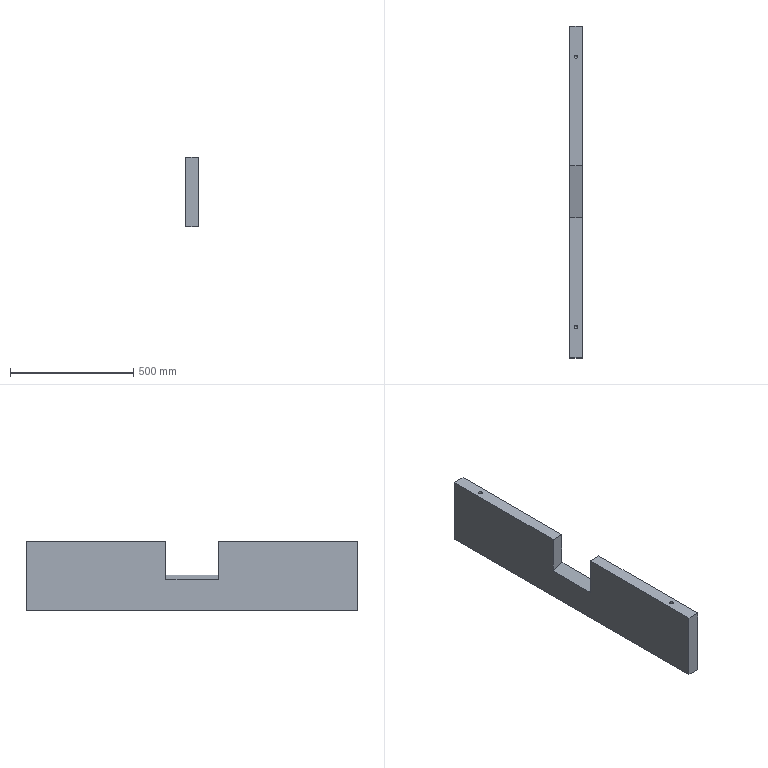Part | NX | features 29 2 | 1 solid | 20 faces | box 50 x 1345 x 280.5 mm | volume 17283100 mm3 | plane 10 | cylinder 5 | cone 5 | commonest cylinder face diameters 14.1 x5
STEP:
#1=CARTESIAN_POINT('',(3647.05,-547.5,-493.5));
#2=VERTEX_POINT('',#1);
#3=CARTESIAN_POINT('',(3640.,-547.5,-493.5));
#4=DIRECTION('',(0.,0.,1.));
#5=DIRECTION('',(1.,0.,0.));
#6=AXIS2_PLACEMENT_3D('',#3,#4,#5);
#7=CIRCLE('',#6,7.05);
#8=EDGE_CURVE('',#2,#2,#7,.T.);
#9=ORIENTED_EDGE('',*,*,#8,.T.);
#10=EDGE_LOOP('',(#9));
#11=FACE_BOUND('',#10,.T.);
#12=CARTESIAN_POINT('',(3615.,672.5,-493.5));
#13=VERTEX_POINT('',#12);
#14=CARTESIAN_POINT('',(3615.,-672.5,-493.5));
#15=VERTEX_POINT('',#14);
#16=CARTESIAN_POINT('',(3615.,193.,-493.5));
#17=DIRECTION('',(0.,-1.,0.));
#18=VECTOR('',#17,1000.);
#19=LINE('',#16,#18);
#20=EDGE_CURVE('',#13,#15,#19,.T.);
#21=ORIENTED_EDGE('',*,*,#20,.F.);
#22=CARTESIAN_POINT('',(3665.,672.5,-493.5));
#23=VERTEX_POINT('',#22);
#24=CARTESIAN_POINT('',(1502.5,672.5,-493.5));
#25=DIRECTION('',(1.,0.,0.));
#26=VECTOR('',#25,1000.);
#27=LINE('',#24,#26);
#28=EDGE_CURVE('',#13,#23,#27,.T.);
#29=ORIENTED_EDGE('',*,*,#28,.T.);
#30=CARTESIAN_POINT('',(3665.,-672.5,-493.5));
#31=VERTEX_POINT('',#30);
#32=CARTESIAN_POINT('',(3665.,193.,-493.5));
#33=DIRECTION('',(0.,1.,0.));
#34=VECTOR('',#33,1000.);
#35=LINE('',#32,#34);
#36=EDGE_CURVE('',#31,#23,#35,.T.);
#37=ORIENTED_EDGE('',*,*,#36,.F.);
#38=CARTESIAN_POINT('',(4005.,-672.5,-493.5));
#39=DIRECTION('',(-1.,0.,0.));
#40=VECTOR('',#39,1000.);
#41=LINE('',#38,#40);
#42=EDGE_CURVE('',#31,#15,#41,.T.);
#43=ORIENTED_EDGE('',*,*,#42,.T.);
#44=EDGE_LOOP('',(#21,#29,#37,#43));
#45=FACE_BOUND('',#44,.T.);
#46=CARTESIAN_POINT('',(3647.05,547.5,-493.5));
#47=VERTEX_POINT('',#46);
#48=CARTESIAN_POINT('',(3640.,547.5,-493.5));
#49=DIRECTION('',(0.,0.,1.));
#50=DIRECTION('',(1.,0.,0.));
#51=AXIS2_PLACEMENT_3D('',#48,#49,#50);
#52=CIRCLE('',#51,7.05);
#53=EDGE_CURVE('',#47,#47,#52,.T.);
#54=ORIENTED_EDGE('',*,*,#53,.T.);
#55=EDGE_LOOP('',(#54));
#56=FACE_BOUND('',#55,.T.);
#57=CARTESIAN_POINT('',(3647.05,0.,-493.5));
#58=VERTEX_POINT('',#57);
#59=CARTESIAN_POINT('',(3640.,0.,-493.5));
#60=DIRECTION('',(0.,0.,1.));
#61=DIRECTION('',(1.,0.,0.));
#62=AXIS2_PLACEMENT_3D('',#59,#60,#61);
#63=CIRCLE('',#62,7.05);
#64=EDGE_CURVE('',#58,#58,#63,.T.);
#65=ORIENTED_EDGE('',*,*,#64,.T.);
#66=EDGE_LOOP('',(#65));
#67=FACE_BOUND('',#66,.T.);
#68=CARTESIAN_POINT('',(1945.,0.,-493.5));
#69=DIRECTION('',(0.,0.,-1.));
#70=DIRECTION('',(1.,0.,0.));
#71=AXIS2_PLACEMENT_3D('',#68,#69,#70);
#72=PLANE('',#71);
#73=ADVANCED_FACE('',(#11,#45,#56,#67),#72,.T.);
#74=CARTESIAN_POINT('',(3665.,-105.579,-213.));
#75=VERTEX_POINT('',#74);
#76=CARTESIAN_POINT('',(3615.,-105.579,-213.));
#77=VERTEX_POINT('',#76);
#78=CARTESIAN_POINT('',(1945.,-105.579,-213.));
#79=DIRECTION('',(-1.,0.,0.));
#80=VECTOR('',#79,1000.);
#81=LINE('',#78,#80);
#82=EDGE_CURVE('',#75,#77,#81,.T.);
#83=ORIENTED_EDGE('',*,*,#82,.T.);
#84=CARTESIAN_POINT('',(3615.,-672.5,-213.));
#85=VERTEX_POINT('',#84);
#86=CARTESIAN_POINT('',(3615.,193.,-213.));
#87=DIRECTION('',(0.,1.,0.));
#88=VECTOR('',#87,1000.);
#89=LINE('',#86,#88);
#90=EDGE_CURVE('',#85,#77,#89,.T.);
#91=ORIENTED_EDGE('',*,*,#90,.F.);
#92=CARTESIAN_POINT('',(3665.,-672.5,-213.));
#93=VERTEX_POINT('',#92);
#94=CARTESIAN_POINT('',(4005.,-672.5,-213.));
#95=DIRECTION('',(1.,0.,0.));
#96=VECTOR('',#95,1000.);
#97=LINE('',#94,#96);
#98=EDGE_CURVE('',#85,#93,#97,.T.);
#99=ORIENTED_EDGE('',*,*,#98,.T.);
#100=CARTESIAN_POINT('',(3665.,193.,-213.));
#101=DIRECTION('',(0.,-1.,0.));
#102=VECTOR('',#101,1000.);
#103=LINE('',#100,#102);
#104=EDGE_CURVE('',#75,#93,#103,.T.);
#105=ORIENTED_EDGE('',*,*,#104,.F.);
#106=EDGE_LOOP('',(#83,#91,#99,#105));
#107=FACE_BOUND('',#106,.T.);
#108=CARTESIAN_POINT('',(3647.05,-547.5,-213.));
#109=VERTEX_POINT('',#108);
#110=CARTESIAN_POINT('',(3640.,-547.5,-213.));
#111=DIRECTION('',(0.,0.,-1.));
#112=DIRECTION('',(1.,0.,0.));
#113=AXIS2_PLACEMENT_3D('',#110,#111,#112);
#114=CIRCLE('',#113,7.05);
#115=EDGE_CURVE('',#109,#109,#114,.T.);
#116=ORIENTED_EDGE('',*,*,#115,.T.);
#117=EDGE_LOOP('',(#116));
#118=FACE_BOUND('',#117,.T.);
#119=CARTESIAN_POINT('',(1945.,0.,-213.));
#120=DIRECTION('',(0.,0.,1.));
#121=DIRECTION('',(-1.,0.,0.));
#122=AXIS2_PLACEMENT_3D('',#119,#120,#121);
#123=PLANE('',#122);
#124=ADVANCED_FACE('',(#107,#118),#123,.T.);
#125=CARTESIAN_POINT('',(3665.,105.421,-213.));
#126=VERTEX_POINT('',#125);
#127=CARTESIAN_POINT('',(3615.,105.421,-213.));
#128=VERTEX_POINT('',#127);
#129=CARTESIAN_POINT('',(3821.81,105.421,-213.));
#130=DIRECTION('',(-1.,0.,0.));
#131=VECTOR('',#130,1000.);
#132=LINE('',#129,#131);
#133=EDGE_CURVE('',#126,#128,#132,.T.);
#134=ORIENTED_EDGE('',*,*,#133,.F.);
#135=CARTESIAN_POINT('',(3665.,672.5,-213.));
#136=VERTEX_POINT('',#135);
#137=CARTESIAN_POINT('',(3665.,193.,-213.));
#138=DIRECTION('',(0.,-1.,0.));
#139=VECTOR('',#138,1000.);
#140=LINE('',#137,#139);
#141=EDGE_CURVE('',#136,#126,#140,.T.);
#142=ORIENTED_EDGE('',*,*,#141,.F.);
#143=CARTESIAN_POINT('',(3615.,672.5,-213.));
#144=VERTEX_POINT('',#143);
#145=CARTESIAN_POINT('',(1502.5,672.5,-213.));
#146=DIRECTION('',(-1.,0.,0.));
#147=VECTOR('',#146,1000.);
#148=LINE('',#145,#147);
#149=EDGE_CURVE('',#136,#144,#148,.T.);
#150=ORIENTED_EDGE('',*,*,#149,.T.);
#151=CARTESIAN_POINT('',(3615.,193.,-213.));
#152=DIRECTION('',(0.,1.,0.));
#153=VECTOR('',#152,1000.);
#154=LINE('',#151,#153);
#155=EDGE_CURVE('',#128,#144,#154,.T.);
#156=ORIENTED_EDGE('',*,*,#155,.F.);
#157=EDGE_LOOP('',(#134,#142,#150,#156));
#158=FACE_BOUND('',#157,.T.);
#159=CARTESIAN_POINT('',(3647.05,547.5,-213.));
#160=VERTEX_POINT('',#159);
#161=CARTESIAN_POINT('',(3640.,547.5,-213.));
#162=DIRECTION('',(0.,0.,-1.));
#163=DIRECTION('',(1.,0.,0.));
#164=AXIS2_PLACEMENT_3D('',#161,#162,#163);
#165=CIRCLE('',#164,7.05);
#166=EDGE_CURVE('',#160,#160,#165,.T.);
#167=ORIENTED_EDGE('',*,*,#166,.T.);
#168=EDGE_LOOP('',(#167));
#169=FACE_BOUND('',#168,.T.);
#170=CARTESIAN_POINT('',(1945.,0.,-213.));
#171=DIRECTION('',(0.,0.,1.));
#172=DIRECTION('',(-1.,0.,0.));
#173=AXIS2_PLACEMENT_3D('',#170,#171,#172);
#174=PLANE('',#173);
#175=ADVANCED_FACE('',(#158,#169),#174,.T.);
#176=ORIENTED_EDGE('',*,*,#90,.T.);
#177=CARTESIAN_POINT('',(3615.,-105.579,-369.004));
#178=VERTEX_POINT('',#177);
#179=CARTESIAN_POINT('',(3615.,-105.579,-205.5));
#180=DIRECTION('',(0.,0.,-1.));
#181=VECTOR('',#180,1000.);
#182=LINE('',#179,#181);
#183=EDGE_CURVE('',#77,#178,#182,.T.);
#184=ORIENTED_EDGE('',*,*,#183,.T.);
#185=CARTESIAN_POINT('',(3615.,105.421,-369.004));
#186=VERTEX_POINT('',#185);
#187=CARTESIAN_POINT('',(3615.,193.,-369.004));
#188=DIRECTION('',(0.,1.,0.));
#189=VECTOR('',#188,1000.);
#190=LINE('',#187,#189);
#191=EDGE_CURVE('',#178,#186,#190,.T.);
#192=ORIENTED_EDGE('',*,*,#191,.T.);
#193=CARTESIAN_POINT('',(3615.,105.421,-205.5));
#194=DIRECTION('',(0.,0.,1.));
#195=VECTOR('',#194,1000.);
#196=LINE('',#193,#195);
#197=EDGE_CURVE('',#186,#128,#196,.T.);
#198=ORIENTED_EDGE('',*,*,#197,.T.);
#199=ORIENTED_EDGE('',*,*,#155,.T.);
#200=CARTESIAN_POINT('',(3615.,672.5,-205.5));
#201=DIRECTION('',(0.,0.,1.));
#202=VECTOR('',#201,1000.);
#203=LINE('',#200,#202);
#204=EDGE_CURVE('',#13,#144,#203,.T.);
#205=ORIENTED_EDGE('',*,*,#204,.F.);
#206=ORIENTED_EDGE('',*,*,#20,.T.);
#207=CARTESIAN_POINT('',(3615.,-672.5,-113.));
#208=DIRECTION('',(0.,0.,1.));
#209=VECTOR('',#208,1000.);
#210=LINE('',#207,#209);
#211=EDGE_CURVE('',#15,#85,#210,.T.);
#212=ORIENTED_EDGE('',*,*,#211,.T.);
#213=EDGE_LOOP('',(#176,#184,#192,#198,#199,#205,#206,#212));
#214=FACE_BOUND('',#213,.T.);
#215=CARTESIAN_POINT('',(3615.,193.,-205.5));
#216=DIRECTION('',(-1.,0.,0.));
#217=DIRECTION('',(0.,0.,1.));
#218=AXIS2_PLACEMENT_3D('',#215,#216,#217);
#219=PLANE('',#218);
#220=ADVANCED_FACE('',(#214),#219,.T.);
#221=ORIENTED_EDGE('',*,*,#28,.F.);
#222=ORIENTED_EDGE('',*,*,#204,.T.);
#223=ORIENTED_EDGE('',*,*,#149,.F.);
#224=CARTESIAN_POINT('',(3665.,672.5,-205.5));
#225=DIRECTION('',(0.,0.,1.));
#226=VECTOR('',#225,1000.);
#227=LINE('',#224,#226);
#228=EDGE_CURVE('',#23,#136,#227,.T.);
#229=ORIENTED_EDGE('',*,*,#228,.F.);
#230=EDGE_LOOP('',(#221,#222,#223,#229));
#231=FACE_BOUND('',#230,.T.);
#232=CARTESIAN_POINT('',(1502.5,672.5,91.));
#233=DIRECTION('',(0.,-1.,0.));
#234=DIRECTION('',(-1.,0.,0.));
#235=AXIS2_PLACEMENT_3D('',#232,#233,#234);
#236=PLANE('',#235);
#237=ADVANCED_FACE('',(#231),#236,.F.);
#238=CARTESIAN_POINT('',(3665.,-105.579,-350.805));
#239=VERTEX_POINT('',#238);
#240=CARTESIAN_POINT('',(3665.,-105.579,-205.5));
#241=DIRECTION('',(0.,0.,1.));
#242=VECTOR('',#241,1000.);
#243=LINE('',#240,#242);
#244=EDGE_CURVE('',#239,#75,#243,.T.);
#245=ORIENTED_EDGE('',*,*,#244,.T.);
#246=ORIENTED_EDGE('',*,*,#104,.T.);
#247=CARTESIAN_POINT('',(3665.,-672.5,-543.5));
#248=DIRECTION('',(0.,0.,1.));
#249=VECTOR('',#248,1000.);
#250=LINE('',#247,#249);
#251=EDGE_CURVE('',#31,#93,#250,.T.);
#252=ORIENTED_EDGE('',*,*,#251,.F.);
#253=ORIENTED_EDGE('',*,*,#36,.T.);
#254=ORIENTED_EDGE('',*,*,#228,.T.);
#255=ORIENTED_EDGE('',*,*,#141,.T.);
#256=CARTESIAN_POINT('',(3665.,105.421,-350.805));
#257=VERTEX_POINT('',#256);
#258=CARTESIAN_POINT('',(3665.,105.421,-205.5));
#259=DIRECTION('',(0.,0.,-1.));
#260=VECTOR('',#259,1000.);
#261=LINE('',#258,#260);
#262=EDGE_CURVE('',#126,#257,#261,.T.);
#263=ORIENTED_EDGE('',*,*,#262,.T.);
#264=CARTESIAN_POINT('',(3665.,193.,-350.805));
#265=DIRECTION('',(0.,-1.,0.));
#266=VECTOR('',#265,1000.);
#267=LINE('',#264,#266);
#268=EDGE_CURVE('',#257,#239,#267,.T.);
#269=ORIENTED_EDGE('',*,*,#268,.T.);
#270=EDGE_LOOP('',(#245,#246,#252,#253,#254,#255,#263,#269));
#271=FACE_BOUND('',#270,.T.);
#272=CARTESIAN_POINT('',(3665.,193.,-205.5));
#273=DIRECTION('',(1.,0.,0.));
#274=DIRECTION('',(0.,0.,-1.));
#275=AXIS2_PLACEMENT_3D('',#272,#273,#274);
#276=PLANE('',#275);
#277=ADVANCED_FACE('',(#271),#276,.T.);
#278=ORIENTED_EDGE('',*,*,#42,.F.);
#279=ORIENTED_EDGE('',*,*,#251,.T.);
#280=ORIENTED_EDGE('',*,*,#98,.F.);
#281=ORIENTED_EDGE('',*,*,#211,.F.);
#282=EDGE_LOOP('',(#278,#279,#280,#281));
#283=FACE_BOUND('',#282,.T.);
#284=CARTESIAN_POINT('',(4005.,-672.5,-113.));
#285=DIRECTION('',(0.,1.,0.));
#286=DIRECTION('',(1.,0.,0.));
#287=AXIS2_PLACEMENT_3D('',#284,#285,#286);
#288=PLANE('',#287);
#289=ADVANCED_FACE('',(#283),#288,.F.);
#290=ORIENTED_EDGE('',*,*,#82,.F.);
#291=ORIENTED_EDGE('',*,*,#244,.F.);
#292=CARTESIAN_POINT('',(3822.494,-105.579,-293.482));
#293=DIRECTION('',(0.9397,0.,0.342));
#294=VECTOR('',#293,1000.);
#295=LINE('',#292,#294);
#296=EDGE_CURVE('',#178,#239,#295,.T.);
#297=ORIENTED_EDGE('',*,*,#296,.F.);
#298=ORIENTED_EDGE('',*,*,#183,.F.);
#299=EDGE_LOOP('',(#290,#291,#297,#298));
#300=FACE_BOUND('',#299,.T.);
#301=CARTESIAN_POINT('',(3821.81,-105.579,-291.603));
#302=DIRECTION('',(0.,1.,0.));
#303=DIRECTION('',(-0.08716,0.,-0.9962));
#304=AXIS2_PLACEMENT_3D('',#301,#302,#303);
#305=PLANE('',#304);
#306=ADVANCED_FACE('',(#300),#305,.T.);
#307=ORIENTED_EDGE('',*,*,#296,.T.);
#308=ORIENTED_EDGE('',*,*,#268,.F.);
#309=CARTESIAN_POINT('',(3822.494,105.421,-293.482));
#310=DIRECTION('',(-0.9397,0.,-0.342));
#311=VECTOR('',#310,1000.);
#312=LINE('',#309,#311);
#313=EDGE_CURVE('',#257,#186,#312,.T.);
#314=ORIENTED_EDGE('',*,*,#313,.T.);
#315=ORIENTED_EDGE('',*,*,#191,.F.);
#316=EDGE_LOOP('',(#307,#308,#314,#315));
#317=FACE_BOUND('',#316,.T.);
#318=CARTESIAN_POINT('',(3822.494,-103.579,-293.482));
#319=DIRECTION('',(-0.342,0.,0.9397));
#320=DIRECTION('',(0.,1.,0.));
#321=AXIS2_PLACEMENT_3D('',#318,#319,#320);
#322=PLANE('',#321);
#323=ADVANCED_FACE('',(#317),#322,.T.);
#324=ORIENTED_EDGE('',*,*,#313,.F.);
#325=ORIENTED_EDGE('',*,*,#262,.F.);
#326=ORIENTED_EDGE('',*,*,#133,.T.);
#327=ORIENTED_EDGE('',*,*,#197,.F.);
#328=EDGE_LOOP('',(#324,#325,#326,#327));
#329=FACE_BOUND('',#328,.T.);
#330=CARTESIAN_POINT('',(3821.81,105.421,-291.603));
#331=DIRECTION('',(0.,-1.,0.));
#332=DIRECTION('',(0.08716,0.,0.9962));
#333=AXIS2_PLACEMENT_3D('',#330,#331,#332);
#334=PLANE('',#333);
#335=ADVANCED_FACE('',(#329),#334,.T.);
#336=CARTESIAN_POINT('',(3632.95,547.5,-249.95));
#337=VERTEX_POINT('',#336);
#338=CARTESIAN_POINT('',(3640.,547.5,-249.95));
#339=DIRECTION('',(0.,0.,-1.));
#340=DIRECTION('',(-1.,0.,0.));
#341=AXIS2_PLACEMENT_3D('',#338,#339,#340);
#342=CIRCLE('',#341,7.05);
#343=EDGE_CURVE('',#337,#337,#342,.T.);
#344=ORIENTED_EDGE('',*,*,#343,.T.);
#345=EDGE_LOOP('',(#344));
#346=FACE_BOUND('',#345,.T.);
#347=ORIENTED_EDGE('',*,*,#166,.F.);
#348=EDGE_LOOP('',(#347));
#349=FACE_BOUND('',#348,.T.);
#350=CARTESIAN_POINT('',(3640.,547.5,-213.));
#351=DIRECTION('',(0.,0.,-1.));
#352=DIRECTION('',(-1.,0.,0.));
#353=AXIS2_PLACEMENT_3D('',#350,#351,#352);
#354=CYLINDRICAL_SURFACE('',#353,7.05);
#355=ADVANCED_FACE('',(#346,#349),#354,.F.);
#356=CARTESIAN_POINT('',(3640.,547.5,-257.));
#357=VERTEX_POINT('',#356);
#358=VERTEX_LOOP('',#357);
#359=FACE_BOUND('',#358,.T.);
#360=ORIENTED_EDGE('',*,*,#343,.F.);
#361=EDGE_LOOP('',(#360));
#362=FACE_BOUND('',#361,.T.);
#363=CARTESIAN_POINT('',(3640.,547.5,-249.95));
#364=DIRECTION('',(0.,0.,1.));
#365=DIRECTION('',(-1.,0.,0.));
#366=AXIS2_PLACEMENT_3D('',#363,#364,#365);
#367=CONICAL_SURFACE('',#366,7.05,0.7854);
#368=ADVANCED_FACE('',(#359,#362),#367,.F.);
#369=CARTESIAN_POINT('',(3632.95,-547.5,-249.95));
#370=VERTEX_POINT('',#369);
#371=CARTESIAN_POINT('',(3640.,-547.5,-249.95));
#372=DIRECTION('',(0.,0.,-1.));
#373=DIRECTION('',(-1.,0.,0.));
#374=AXIS2_PLACEMENT_3D('',#371,#372,#373);
#375=CIRCLE('',#374,7.05);
#376=EDGE_CURVE('',#370,#370,#375,.T.);
#377=ORIENTED_EDGE('',*,*,#376,.T.);
#378=EDGE_LOOP('',(#377));
#379=FACE_BOUND('',#378,.T.);
#380=ORIENTED_EDGE('',*,*,#115,.F.);
#381=EDGE_LOOP('',(#380));
#382=FACE_BOUND('',#381,.T.);
#383=CARTESIAN_POINT('',(3640.,-547.5,-213.));
#384=DIRECTION('',(0.,0.,-1.));
#385=DIRECTION('',(-1.,0.,0.));
#386=AXIS2_PLACEMENT_3D('',#383,#384,#385);
#387=CYLINDRICAL_SURFACE('',#386,7.05);
#388=ADVANCED_FACE('',(#379,#382),#387,.F.);
#389=CARTESIAN_POINT('',(3640.,-547.5,-257.));
#390=VERTEX_POINT('',#389);
#391=VERTEX_LOOP('',#390);
#392=FACE_BOUND('',#391,.T.);
#393=ORIENTED_EDGE('',*,*,#376,.F.);
#394=EDGE_LOOP('',(#393));
#395=FACE_BOUND('',#394,.T.);
#396=CARTESIAN_POINT('',(3640.,-547.5,-249.95));
#397=DIRECTION('',(0.,0.,1.));
#398=DIRECTION('',(-1.,0.,0.));
#399=AXIS2_PLACEMENT_3D('',#396,#397,#398);
#400=CONICAL_SURFACE('',#399,7.05,0.7854);
#401=ADVANCED_FACE('',(#392,#395),#400,.F.);
#402=CARTESIAN_POINT('',(3647.05,547.5,-456.55));
#403=VERTEX_POINT('',#402);
#404=CARTESIAN_POINT('',(3640.,547.5,-456.55));
#405=DIRECTION('',(0.,0.,1.));
#406=DIRECTION('',(1.,0.,0.));
#407=AXIS2_PLACEMENT_3D('',#404,#405,#406);
#408=CIRCLE('',#407,7.05);
#409=EDGE_CURVE('',#403,#403,#408,.T.);
#410=ORIENTED_EDGE('',*,*,#409,.T.);
#411=EDGE_LOOP('',(#410));
#412=FACE_BOUND('',#411,.T.);
#413=ORIENTED_EDGE('',*,*,#53,.F.);
#414=EDGE_LOOP('',(#413));
#415=FACE_BOUND('',#414,.T.);
#416=CARTESIAN_POINT('',(3640.,547.5,-493.5));
#417=DIRECTION('',(0.,0.,1.));
#418=DIRECTION('',(-1.,0.,0.));
#419=AXIS2_PLACEMENT_3D('',#416,#417,#418);
#420=CYLINDRICAL_SURFACE('',#419,7.05);
#421=ADVANCED_FACE('',(#412,#415),#420,.F.);
#422=CARTESIAN_POINT('',(3640.,547.5,-449.5));
#423=VERTEX_POINT('',#422);
#424=VERTEX_LOOP('',#423);
#425=FACE_BOUND('',#424,.T.);
#426=ORIENTED_EDGE('',*,*,#409,.F.);
#427=EDGE_LOOP('',(#426));
#428=FACE_BOUND('',#427,.T.);
#429=CARTESIAN_POINT('',(3640.,547.5,-456.55));
#430=DIRECTION('',(0.,0.,-1.));
#431=DIRECTION('',(1.,0.,0.));
#432=AXIS2_PLACEMENT_3D('',#429,#430,#431);
#433=CONICAL_SURFACE('',#432,7.05,0.7854);
#434=ADVANCED_FACE('',(#425,#428),#433,.F.);
#435=CARTESIAN_POINT('',(3647.05,-547.5,-456.55));
#436=VERTEX_POINT('',#435);
#437=CARTESIAN_POINT('',(3640.,-547.5,-456.55));
#438=DIRECTION('',(0.,0.,1.));
#439=DIRECTION('',(1.,0.,0.));
#440=AXIS2_PLACEMENT_3D('',#437,#438,#439);
#441=CIRCLE('',#440,7.05);
#442=EDGE_CURVE('',#436,#436,#441,.T.);
#443=ORIENTED_EDGE('',*,*,#442,.T.);
#444=EDGE_LOOP('',(#443));
#445=FACE_BOUND('',#444,.T.);
#446=ORIENTED_EDGE('',*,*,#8,.F.);
#447=EDGE_LOOP('',(#446));
#448=FACE_BOUND('',#447,.T.);
#449=CARTESIAN_POINT('',(3640.,-547.5,-493.5));
#450=DIRECTION('',(0.,0.,1.));
#451=DIRECTION('',(-1.,0.,0.));
#452=AXIS2_PLACEMENT_3D('',#449,#450,#451);
#453=CYLINDRICAL_SURFACE('',#452,7.05);
#454=ADVANCED_FACE('',(#445,#448),#453,.F.);
#455=CARTESIAN_POINT('',(3640.,-547.5,-449.5));
#456=VERTEX_POINT('',#455);
#457=VERTEX_LOOP('',#456);
#458=FACE_BOUND('',#457,.T.);
#459=ORIENTED_EDGE('',*,*,#442,.F.);
#460=EDGE_LOOP('',(#459));
#461=FACE_BOUND('',#460,.T.);
#462=CARTESIAN_POINT('',(3640.,-547.5,-456.55));
#463=DIRECTION('',(0.,0.,-1.));
#464=DIRECTION('',(1.,0.,0.));
#465=AXIS2_PLACEMENT_3D('',#462,#463,#464);
#466=CONICAL_SURFACE('',#465,7.05,0.7854);
#467=ADVANCED_FACE('',(#458,#461),#466,.F.);
#468=CARTESIAN_POINT('',(3647.05,0.,-456.55));
#469=VERTEX_POINT('',#468);
#470=CARTESIAN_POINT('',(3640.,0.,-456.55));
#471=DIRECTION('',(0.,0.,1.));
#472=DIRECTION('',(1.,0.,0.));
#473=AXIS2_PLACEMENT_3D('',#470,#471,#472);
#474=CIRCLE('',#473,7.05);
#475=EDGE_CURVE('',#469,#469,#474,.T.);
#476=ORIENTED_EDGE('',*,*,#475,.T.);
#477=EDGE_LOOP('',(#476));
#478=FACE_BOUND('',#477,.T.);
#479=ORIENTED_EDGE('',*,*,#64,.F.);
#480=EDGE_LOOP('',(#479));
#481=FACE_BOUND('',#480,.T.);
#482=CARTESIAN_POINT('',(3640.,0.,-493.5));
#483=DIRECTION('',(0.,0.,1.));
#484=DIRECTION('',(-1.,0.,0.));
#485=AXIS2_PLACEMENT_3D('',#482,#483,#484);
#486=CYLINDRICAL_SURFACE('',#485,7.05);
#487=ADVANCED_FACE('',(#478,#481),#486,.F.);
#488=CARTESIAN_POINT('',(3640.,0.,-449.5));
#489=VERTEX_POINT('',#488);
#490=VERTEX_LOOP('',#489);
#491=FACE_BOUND('',#490,.T.);
#492=ORIENTED_EDGE('',*,*,#475,.F.);
#493=EDGE_LOOP('',(#492));
#494=FACE_BOUND('',#493,.T.);
#495=CARTESIAN_POINT('',(3640.,0.,-456.55));
#496=DIRECTION('',(0.,0.,-1.));
#497=DIRECTION('',(1.,0.,0.));
#498=AXIS2_PLACEMENT_3D('',#495,#496,#497);
#499=CONICAL_SURFACE('',#498,7.05,0.7854);
#500=ADVANCED_FACE('',(#491,#494),#499,.F.);
#501=CLOSED_SHELL('',(#73,#124,#175,#220,#237,#277,#289,#306,#323,#335,#355,#368,#388,#401,#421,#434,#454,#467,#487,#500));
#502=MANIFOLD_SOLID_BREP('',#501);
#503=(LENGTH_UNIT()NAMED_UNIT(*)SI_UNIT(.MILLI.,.METRE.));
#504=UNCERTAINTY_MEASURE_WITH_UNIT(LENGTH_MEASURE(0.00001),#503,'','');
#505=(NAMED_UNIT(*)PLANE_ANGLE_UNIT()SI_UNIT($,.RADIAN.));
#506=(NAMED_UNIT(*)SI_UNIT($,.STERADIAN.)SOLID_ANGLE_UNIT());
#507=(GEOMETRIC_REPRESENTATION_CONTEXT(3)GLOBAL_UNCERTAINTY_ASSIGNED_CONTEXT((#504))GLOBAL_UNIT_ASSIGNED_CONTEXT((#503,#505,#506))REPRESENTATION_CONTEXT('',''));
#508=ADVANCED_BREP_SHAPE_REPRESENTATION('',(#502),#507);